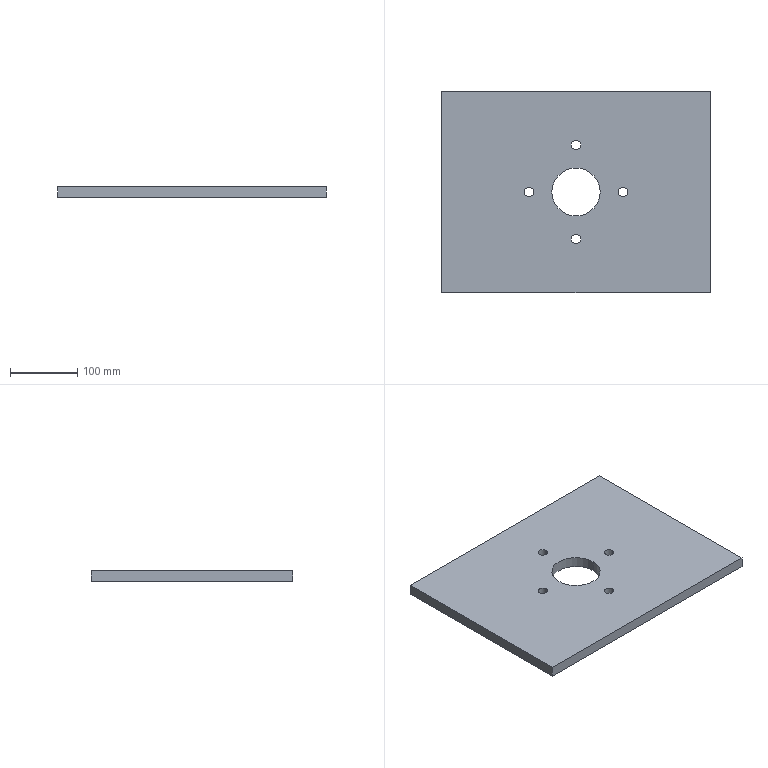Part | STEP file | 15-Steel plate | 1 solid | 16 faces | box 400 x 300 x 16 mm | volume 1845004 mm3 | cylinder 10 | plane 6 | commonest cylinder face diameters 14 x8 72 x2
STEP:
#1=CARTESIAN_POINT('',(0.,0.,0.));
#2=DIRECTION('',(0.,0.,1.));
#3=DIRECTION('',(1.,0.,0.));
#4=AXIS2_PLACEMENT_3D('',#1,#2,#3);
#5=CARTESIAN_POINT('',(207.,-80.,0.));
#6=VERTEX_POINT('',#5);
#7=CARTESIAN_POINT('',(207.,-80.,16.));
#8=VERTEX_POINT('',#7);
#9=CARTESIAN_POINT('',(207.,-80.,16.));
#10=DIRECTION('',(0.,0.,1.));
#11=VECTOR('',#10,1.);
#12=LINE('',#9,#11);
#13=CARTESIAN_POINT('',(200.,-80.,16.));
#14=DIRECTION('',(0.,0.,1.));
#15=DIRECTION('',(1.,0.,0.));
#16=AXIS2_PLACEMENT_3D('',#13,#14,#15);
#17=CYLINDRICAL_SURFACE('',#16,7.);
#18=CARTESIAN_POINT('',(6.283,0.));
#19=DIRECTION('',(0.,1.));
#20=VECTOR('',#19,1.);
#21=LINE('',#18,#20);
#22=(GEOMETRIC_REPRESENTATION_CONTEXT(2)PARAMETRIC_REPRESENTATION_CONTEXT()REPRESENTATION_CONTEXT('',''));
#23=DEFINITIONAL_REPRESENTATION('',(#21),#22);
#24=PCURVE('',#17,#23);
#25=CARTESIAN_POINT('',(200.,-80.,16.));
#26=DIRECTION('',(0.,0.,1.));
#27=DIRECTION('',(1.,0.,0.));
#28=AXIS2_PLACEMENT_3D('',#25,#26,#27);
#29=CYLINDRICAL_SURFACE('',#28,7.);
#30=CARTESIAN_POINT('',(0.,0.));
#31=DIRECTION('',(0.,1.));
#32=VECTOR('',#31,1.);
#33=LINE('',#30,#32);
#34=(GEOMETRIC_REPRESENTATION_CONTEXT(2)PARAMETRIC_REPRESENTATION_CONTEXT()REPRESENTATION_CONTEXT('',''));
#35=DEFINITIONAL_REPRESENTATION('',(#33),#34);
#36=PCURVE('',#29,#35);
#37=SURFACE_CURVE('',#12,(#24,#36),.PCURVE_S1.);
#38=EDGE_CURVE('',#6,#8,#37,.T.);
#39=ORIENTED_EDGE('',*,*,#38,.T.);
#40=CARTESIAN_POINT('',(193.,-80.,16.));
#41=VERTEX_POINT('',#40);
#42=CARTESIAN_POINT('',(200.,-80.,16.));
#43=DIRECTION('',(0.,0.,1.));
#44=DIRECTION('',(1.,0.,0.));
#45=AXIS2_PLACEMENT_3D('',#42,#43,#44);
#46=CIRCLE('',#45,7.);
#47=CARTESIAN_POINT('',(0.,0.));
#48=DIRECTION('',(1.,0.));
#49=VECTOR('',#48,1.);
#50=LINE('',#47,#49);
#51=(GEOMETRIC_REPRESENTATION_CONTEXT(2)PARAMETRIC_REPRESENTATION_CONTEXT()REPRESENTATION_CONTEXT('',''));
#52=DEFINITIONAL_REPRESENTATION('',(#50),#51);
#53=PCURVE('',#17,#52);
#54=CARTESIAN_POINT('',(0.,0.,16.));
#55=DIRECTION('',(0.,0.,1.));
#56=DIRECTION('',(1.,0.,0.));
#57=AXIS2_PLACEMENT_3D('',#54,#55,#56);
#58=PLANE('',#57);
#59=CARTESIAN_POINT('',(200.,-80.));
#60=DIRECTION('',(1.,0.));
#61=AXIS2_PLACEMENT_2D('',#59,#60);
#62=CIRCLE('',#61,7.);
#63=(GEOMETRIC_REPRESENTATION_CONTEXT(2)PARAMETRIC_REPRESENTATION_CONTEXT()REPRESENTATION_CONTEXT('',''));
#64=DEFINITIONAL_REPRESENTATION('',(#62),#63);
#65=PCURVE('',#58,#64);
#66=SURFACE_CURVE('',#46,(#53,#65),.PCURVE_S1.);
#67=EDGE_CURVE('',#41,#8,#66,.T.);
#68=ORIENTED_EDGE('',*,*,#67,.F.);
#69=CARTESIAN_POINT('',(193.,-80.,0.));
#70=VERTEX_POINT('',#69);
#71=CARTESIAN_POINT('',(193.,-80.,16.));
#72=DIRECTION('',(0.,0.,1.));
#73=VECTOR('',#72,1.);
#74=LINE('',#71,#73);
#75=CARTESIAN_POINT('',(3.142,0.));
#76=DIRECTION('',(0.,1.));
#77=VECTOR('',#76,1.);
#78=LINE('',#75,#77);
#79=(GEOMETRIC_REPRESENTATION_CONTEXT(2)PARAMETRIC_REPRESENTATION_CONTEXT()REPRESENTATION_CONTEXT('',''));
#80=DEFINITIONAL_REPRESENTATION('',(#78),#79);
#81=PCURVE('',#17,#80);
#82=CARTESIAN_POINT('',(3.142,0.));
#83=DIRECTION('',(0.,1.));
#84=VECTOR('',#83,1.);
#85=LINE('',#82,#84);
#86=(GEOMETRIC_REPRESENTATION_CONTEXT(2)PARAMETRIC_REPRESENTATION_CONTEXT()REPRESENTATION_CONTEXT('',''));
#87=DEFINITIONAL_REPRESENTATION('',(#85),#86);
#88=PCURVE('',#29,#87);
#89=SURFACE_CURVE('',#74,(#81,#88),.PCURVE_S1.);
#90=EDGE_CURVE('',#70,#41,#89,.T.);
#91=ORIENTED_EDGE('',*,*,#90,.F.);
#92=CARTESIAN_POINT('',(200.,-80.,0.));
#93=DIRECTION('',(0.,0.,1.));
#94=DIRECTION('',(1.,0.,0.));
#95=AXIS2_PLACEMENT_3D('',#92,#93,#94);
#96=CIRCLE('',#95,7.);
#97=CARTESIAN_POINT('',(0.,-16.));
#98=DIRECTION('',(1.,0.));
#99=VECTOR('',#98,1.);
#100=LINE('',#97,#99);
#101=(GEOMETRIC_REPRESENTATION_CONTEXT(2)PARAMETRIC_REPRESENTATION_CONTEXT()REPRESENTATION_CONTEXT('',''));
#102=DEFINITIONAL_REPRESENTATION('',(#100),#101);
#103=PCURVE('',#17,#102);
#104=CARTESIAN_POINT('',(0.,0.,0.));
#105=DIRECTION('',(0.,0.,1.));
#106=DIRECTION('',(1.,0.,0.));
#107=AXIS2_PLACEMENT_3D('',#104,#105,#106);
#108=PLANE('',#107);
#109=CARTESIAN_POINT('',(200.,-80.));
#110=DIRECTION('',(1.,0.));
#111=AXIS2_PLACEMENT_2D('',#109,#110);
#112=CIRCLE('',#111,7.);
#113=(GEOMETRIC_REPRESENTATION_CONTEXT(2)PARAMETRIC_REPRESENTATION_CONTEXT()REPRESENTATION_CONTEXT('',''));
#114=DEFINITIONAL_REPRESENTATION('',(#112),#113);
#115=PCURVE('',#108,#114);
#116=SURFACE_CURVE('',#96,(#103,#115),.PCURVE_S1.);
#117=EDGE_CURVE('',#70,#6,#116,.T.);
#118=ORIENTED_EDGE('',*,*,#117,.T.);
#119=EDGE_LOOP('',(#39,#68,#91,#118));
#120=FACE_BOUND('',#119,.F.);
#121=ADVANCED_FACE('',(#120),#17,.F.);
#122=CARTESIAN_POINT('',(207.,-220.,0.));
#123=VERTEX_POINT('',#122);
#124=CARTESIAN_POINT('',(207.,-220.,16.));
#125=VERTEX_POINT('',#124);
#126=CARTESIAN_POINT('',(207.,-220.,16.));
#127=DIRECTION('',(0.,0.,1.));
#128=VECTOR('',#127,1.);
#129=LINE('',#126,#128);
#130=CARTESIAN_POINT('',(200.,-220.,16.));
#131=DIRECTION('',(0.,0.,1.));
#132=DIRECTION('',(1.,0.,0.));
#133=AXIS2_PLACEMENT_3D('',#130,#131,#132);
#134=CYLINDRICAL_SURFACE('',#133,7.);
#135=CARTESIAN_POINT('',(6.283,0.));
#136=DIRECTION('',(0.,1.));
#137=VECTOR('',#136,1.);
#138=LINE('',#135,#137);
#139=(GEOMETRIC_REPRESENTATION_CONTEXT(2)PARAMETRIC_REPRESENTATION_CONTEXT()REPRESENTATION_CONTEXT('',''));
#140=DEFINITIONAL_REPRESENTATION('',(#138),#139);
#141=PCURVE('',#134,#140);
#142=CARTESIAN_POINT('',(200.,-220.,16.));
#143=DIRECTION('',(0.,0.,1.));
#144=DIRECTION('',(1.,0.,0.));
#145=AXIS2_PLACEMENT_3D('',#142,#143,#144);
#146=CYLINDRICAL_SURFACE('',#145,7.);
#147=CARTESIAN_POINT('',(0.,0.));
#148=DIRECTION('',(0.,1.));
#149=VECTOR('',#148,1.);
#150=LINE('',#147,#149);
#151=(GEOMETRIC_REPRESENTATION_CONTEXT(2)PARAMETRIC_REPRESENTATION_CONTEXT()REPRESENTATION_CONTEXT('',''));
#152=DEFINITIONAL_REPRESENTATION('',(#150),#151);
#153=PCURVE('',#146,#152);
#154=SURFACE_CURVE('',#129,(#141,#153),.PCURVE_S1.);
#155=EDGE_CURVE('',#123,#125,#154,.T.);
#156=ORIENTED_EDGE('',*,*,#155,.T.);
#157=CARTESIAN_POINT('',(193.,-220.,16.));
#158=VERTEX_POINT('',#157);
#159=CARTESIAN_POINT('',(200.,-220.,16.));
#160=DIRECTION('',(0.,0.,1.));
#161=DIRECTION('',(1.,0.,0.));
#162=AXIS2_PLACEMENT_3D('',#159,#160,#161);
#163=CIRCLE('',#162,7.);
#164=CARTESIAN_POINT('',(0.,0.));
#165=DIRECTION('',(1.,0.));
#166=VECTOR('',#165,1.);
#167=LINE('',#164,#166);
#168=(GEOMETRIC_REPRESENTATION_CONTEXT(2)PARAMETRIC_REPRESENTATION_CONTEXT()REPRESENTATION_CONTEXT('',''));
#169=DEFINITIONAL_REPRESENTATION('',(#167),#168);
#170=PCURVE('',#134,#169);
#171=CARTESIAN_POINT('',(200.,-220.));
#172=DIRECTION('',(1.,0.));
#173=AXIS2_PLACEMENT_2D('',#171,#172);
#174=CIRCLE('',#173,7.);
#175=(GEOMETRIC_REPRESENTATION_CONTEXT(2)PARAMETRIC_REPRESENTATION_CONTEXT()REPRESENTATION_CONTEXT('',''));
#176=DEFINITIONAL_REPRESENTATION('',(#174),#175);
#177=PCURVE('',#58,#176);
#178=SURFACE_CURVE('',#163,(#170,#177),.PCURVE_S1.);
#179=EDGE_CURVE('',#158,#125,#178,.T.);
#180=ORIENTED_EDGE('',*,*,#179,.F.);
#181=CARTESIAN_POINT('',(193.,-220.,0.));
#182=VERTEX_POINT('',#181);
#183=CARTESIAN_POINT('',(193.,-220.,16.));
#184=DIRECTION('',(0.,0.,1.));
#185=VECTOR('',#184,1.);
#186=LINE('',#183,#185);
#187=CARTESIAN_POINT('',(3.142,0.));
#188=DIRECTION('',(0.,1.));
#189=VECTOR('',#188,1.);
#190=LINE('',#187,#189);
#191=(GEOMETRIC_REPRESENTATION_CONTEXT(2)PARAMETRIC_REPRESENTATION_CONTEXT()REPRESENTATION_CONTEXT('',''));
#192=DEFINITIONAL_REPRESENTATION('',(#190),#191);
#193=PCURVE('',#134,#192);
#194=CARTESIAN_POINT('',(3.142,0.));
#195=DIRECTION('',(0.,1.));
#196=VECTOR('',#195,1.);
#197=LINE('',#194,#196);
#198=(GEOMETRIC_REPRESENTATION_CONTEXT(2)PARAMETRIC_REPRESENTATION_CONTEXT()REPRESENTATION_CONTEXT('',''));
#199=DEFINITIONAL_REPRESENTATION('',(#197),#198);
#200=PCURVE('',#146,#199);
#201=SURFACE_CURVE('',#186,(#193,#200),.PCURVE_S1.);
#202=EDGE_CURVE('',#182,#158,#201,.T.);
#203=ORIENTED_EDGE('',*,*,#202,.F.);
#204=CARTESIAN_POINT('',(200.,-220.,0.));
#205=DIRECTION('',(0.,0.,1.));
#206=DIRECTION('',(1.,0.,0.));
#207=AXIS2_PLACEMENT_3D('',#204,#205,#206);
#208=CIRCLE('',#207,7.);
#209=CARTESIAN_POINT('',(0.,-16.));
#210=DIRECTION('',(1.,0.));
#211=VECTOR('',#210,1.);
#212=LINE('',#209,#211);
#213=(GEOMETRIC_REPRESENTATION_CONTEXT(2)PARAMETRIC_REPRESENTATION_CONTEXT()REPRESENTATION_CONTEXT('',''));
#214=DEFINITIONAL_REPRESENTATION('',(#212),#213);
#215=PCURVE('',#134,#214);
#216=CARTESIAN_POINT('',(200.,-220.));
#217=DIRECTION('',(1.,0.));
#218=AXIS2_PLACEMENT_2D('',#216,#217);
#219=CIRCLE('',#218,7.);
#220=(GEOMETRIC_REPRESENTATION_CONTEXT(2)PARAMETRIC_REPRESENTATION_CONTEXT()REPRESENTATION_CONTEXT('',''));
#221=DEFINITIONAL_REPRESENTATION('',(#219),#220);
#222=PCURVE('',#108,#221);
#223=SURFACE_CURVE('',#208,(#215,#222),.PCURVE_S1.);
#224=EDGE_CURVE('',#182,#123,#223,.T.);
#225=ORIENTED_EDGE('',*,*,#224,.T.);
#226=EDGE_LOOP('',(#156,#180,#203,#225));
#227=FACE_BOUND('',#226,.F.);
#228=ADVANCED_FACE('',(#227),#134,.F.);
#229=CARTESIAN_POINT('',(277.,-150.,0.));
#230=VERTEX_POINT('',#229);
#231=CARTESIAN_POINT('',(277.,-150.,16.));
#232=VERTEX_POINT('',#231);
#233=CARTESIAN_POINT('',(277.,-150.,16.));
#234=DIRECTION('',(0.,0.,1.));
#235=VECTOR('',#234,1.);
#236=LINE('',#233,#235);
#237=CARTESIAN_POINT('',(270.,-150.,16.));
#238=DIRECTION('',(0.,0.,1.));
#239=DIRECTION('',(1.,0.,0.));
#240=AXIS2_PLACEMENT_3D('',#237,#238,#239);
#241=CYLINDRICAL_SURFACE('',#240,7.);
#242=CARTESIAN_POINT('',(6.283,0.));
#243=DIRECTION('',(0.,1.));
#244=VECTOR('',#243,1.);
#245=LINE('',#242,#244);
#246=(GEOMETRIC_REPRESENTATION_CONTEXT(2)PARAMETRIC_REPRESENTATION_CONTEXT()REPRESENTATION_CONTEXT('',''));
#247=DEFINITIONAL_REPRESENTATION('',(#245),#246);
#248=PCURVE('',#241,#247);
#249=CARTESIAN_POINT('',(270.,-150.,16.));
#250=DIRECTION('',(0.,0.,1.));
#251=DIRECTION('',(1.,0.,0.));
#252=AXIS2_PLACEMENT_3D('',#249,#250,#251);
#253=CYLINDRICAL_SURFACE('',#252,7.);
#254=CARTESIAN_POINT('',(0.,0.));
#255=DIRECTION('',(0.,1.));
#256=VECTOR('',#255,1.);
#257=LINE('',#254,#256);
#258=(GEOMETRIC_REPRESENTATION_CONTEXT(2)PARAMETRIC_REPRESENTATION_CONTEXT()REPRESENTATION_CONTEXT('',''));
#259=DEFINITIONAL_REPRESENTATION('',(#257),#258);
#260=PCURVE('',#253,#259);
#261=SURFACE_CURVE('',#236,(#248,#260),.PCURVE_S1.);
#262=EDGE_CURVE('',#230,#232,#261,.T.);
#263=ORIENTED_EDGE('',*,*,#262,.T.);
#264=CARTESIAN_POINT('',(263.,-150.,16.));
#265=VERTEX_POINT('',#264);
#266=CARTESIAN_POINT('',(270.,-150.,16.));
#267=DIRECTION('',(0.,0.,1.));
#268=DIRECTION('',(1.,0.,0.));
#269=AXIS2_PLACEMENT_3D('',#266,#267,#268);
#270=CIRCLE('',#269,7.);
#271=CARTESIAN_POINT('',(0.,0.));
#272=DIRECTION('',(1.,0.));
#273=VECTOR('',#272,1.);
#274=LINE('',#271,#273);
#275=(GEOMETRIC_REPRESENTATION_CONTEXT(2)PARAMETRIC_REPRESENTATION_CONTEXT()REPRESENTATION_CONTEXT('',''));
#276=DEFINITIONAL_REPRESENTATION('',(#274),#275);
#277=PCURVE('',#241,#276);
#278=CARTESIAN_POINT('',(270.,-150.));
#279=DIRECTION('',(1.,0.));
#280=AXIS2_PLACEMENT_2D('',#278,#279);
#281=CIRCLE('',#280,7.);
#282=(GEOMETRIC_REPRESENTATION_CONTEXT(2)PARAMETRIC_REPRESENTATION_CONTEXT()REPRESENTATION_CONTEXT('',''));
#283=DEFINITIONAL_REPRESENTATION('',(#281),#282);
#284=PCURVE('',#58,#283);
#285=SURFACE_CURVE('',#270,(#277,#284),.PCURVE_S1.);
#286=EDGE_CURVE('',#265,#232,#285,.T.);
#287=ORIENTED_EDGE('',*,*,#286,.F.);
#288=CARTESIAN_POINT('',(263.,-150.,0.));
#289=VERTEX_POINT('',#288);
#290=CARTESIAN_POINT('',(263.,-150.,16.));
#291=DIRECTION('',(0.,0.,1.));
#292=VECTOR('',#291,1.);
#293=LINE('',#290,#292);
#294=CARTESIAN_POINT('',(3.142,0.));
#295=DIRECTION('',(0.,1.));
#296=VECTOR('',#295,1.);
#297=LINE('',#294,#296);
#298=(GEOMETRIC_REPRESENTATION_CONTEXT(2)PARAMETRIC_REPRESENTATION_CONTEXT()REPRESENTATION_CONTEXT('',''));
#299=DEFINITIONAL_REPRESENTATION('',(#297),#298);
#300=PCURVE('',#241,#299);
#301=CARTESIAN_POINT('',(3.142,0.));
#302=DIRECTION('',(0.,1.));
#303=VECTOR('',#302,1.);
#304=LINE('',#301,#303);
#305=(GEOMETRIC_REPRESENTATION_CONTEXT(2)PARAMETRIC_REPRESENTATION_CONTEXT()REPRESENTATION_CONTEXT('',''));
#306=DEFINITIONAL_REPRESENTATION('',(#304),#305);
#307=PCURVE('',#253,#306);
#308=SURFACE_CURVE('',#293,(#300,#307),.PCURVE_S1.);
#309=EDGE_CURVE('',#289,#265,#308,.T.);
#310=ORIENTED_EDGE('',*,*,#309,.F.);
#311=CARTESIAN_POINT('',(270.,-150.,0.));
#312=DIRECTION('',(0.,0.,1.));
#313=DIRECTION('',(1.,0.,0.));
#314=AXIS2_PLACEMENT_3D('',#311,#312,#313);
#315=CIRCLE('',#314,7.);
#316=CARTESIAN_POINT('',(0.,-16.));
#317=DIRECTION('',(1.,0.));
#318=VECTOR('',#317,1.);
#319=LINE('',#316,#318);
#320=(GEOMETRIC_REPRESENTATION_CONTEXT(2)PARAMETRIC_REPRESENTATION_CONTEXT()REPRESENTATION_CONTEXT('',''));
#321=DEFINITIONAL_REPRESENTATION('',(#319),#320);
#322=PCURVE('',#241,#321);
#323=CARTESIAN_POINT('',(270.,-150.));
#324=DIRECTION('',(1.,0.));
#325=AXIS2_PLACEMENT_2D('',#323,#324);
#326=CIRCLE('',#325,7.);
#327=(GEOMETRIC_REPRESENTATION_CONTEXT(2)PARAMETRIC_REPRESENTATION_CONTEXT()REPRESENTATION_CONTEXT('',''));
#328=DEFINITIONAL_REPRESENTATION('',(#326),#327);
#329=PCURVE('',#108,#328);
#330=SURFACE_CURVE('',#315,(#322,#329),.PCURVE_S1.);
#331=EDGE_CURVE('',#289,#230,#330,.T.);
#332=ORIENTED_EDGE('',*,*,#331,.T.);
#333=EDGE_LOOP('',(#263,#287,#310,#332));
#334=FACE_BOUND('',#333,.F.);
#335=ADVANCED_FACE('',(#334),#241,.F.);
#336=CARTESIAN_POINT('',(137.,-150.,0.));
#337=VERTEX_POINT('',#336);
#338=CARTESIAN_POINT('',(137.,-150.,16.));
#339=VERTEX_POINT('',#338);
#340=CARTESIAN_POINT('',(137.,-150.,16.));
#341=DIRECTION('',(0.,0.,1.));
#342=VECTOR('',#341,1.);
#343=LINE('',#340,#342);
#344=CARTESIAN_POINT('',(130.,-150.,16.));
#345=DIRECTION('',(0.,0.,1.));
#346=DIRECTION('',(1.,0.,0.));
#347=AXIS2_PLACEMENT_3D('',#344,#345,#346);
#348=CYLINDRICAL_SURFACE('',#347,7.);
#349=CARTESIAN_POINT('',(6.283,0.));
#350=DIRECTION('',(0.,1.));
#351=VECTOR('',#350,1.);
#352=LINE('',#349,#351);
#353=(GEOMETRIC_REPRESENTATION_CONTEXT(2)PARAMETRIC_REPRESENTATION_CONTEXT()REPRESENTATION_CONTEXT('',''));
#354=DEFINITIONAL_REPRESENTATION('',(#352),#353);
#355=PCURVE('',#348,#354);
#356=CARTESIAN_POINT('',(130.,-150.,16.));
#357=DIRECTION('',(0.,0.,1.));
#358=DIRECTION('',(1.,0.,0.));
#359=AXIS2_PLACEMENT_3D('',#356,#357,#358);
#360=CYLINDRICAL_SURFACE('',#359,7.);
#361=CARTESIAN_POINT('',(0.,0.));
#362=DIRECTION('',(0.,1.));
#363=VECTOR('',#362,1.);
#364=LINE('',#361,#363);
#365=(GEOMETRIC_REPRESENTATION_CONTEXT(2)PARAMETRIC_REPRESENTATION_CONTEXT()REPRESENTATION_CONTEXT('',''));
#366=DEFINITIONAL_REPRESENTATION('',(#364),#365);
#367=PCURVE('',#360,#366);
#368=SURFACE_CURVE('',#343,(#355,#367),.PCURVE_S1.);
#369=EDGE_CURVE('',#337,#339,#368,.T.);
#370=ORIENTED_EDGE('',*,*,#369,.T.);
#371=CARTESIAN_POINT('',(123.,-150.,16.));
#372=VERTEX_POINT('',#371);
#373=CARTESIAN_POINT('',(130.,-150.,16.));
#374=DIRECTION('',(0.,0.,1.));
#375=DIRECTION('',(1.,0.,0.));
#376=AXIS2_PLACEMENT_3D('',#373,#374,#375);
#377=CIRCLE('',#376,7.);
#378=CARTESIAN_POINT('',(0.,0.));
#379=DIRECTION('',(1.,0.));
#380=VECTOR('',#379,1.);
#381=LINE('',#378,#380);
#382=(GEOMETRIC_REPRESENTATION_CONTEXT(2)PARAMETRIC_REPRESENTATION_CONTEXT()REPRESENTATION_CONTEXT('',''));
#383=DEFINITIONAL_REPRESENTATION('',(#381),#382);
#384=PCURVE('',#348,#383);
#385=CARTESIAN_POINT('',(130.,-150.));
#386=DIRECTION('',(1.,0.));
#387=AXIS2_PLACEMENT_2D('',#385,#386);
#388=CIRCLE('',#387,7.);
#389=(GEOMETRIC_REPRESENTATION_CONTEXT(2)PARAMETRIC_REPRESENTATION_CONTEXT()REPRESENTATION_CONTEXT('',''));
#390=DEFINITIONAL_REPRESENTATION('',(#388),#389);
#391=PCURVE('',#58,#390);
#392=SURFACE_CURVE('',#377,(#384,#391),.PCURVE_S1.);
#393=EDGE_CURVE('',#372,#339,#392,.T.);
#394=ORIENTED_EDGE('',*,*,#393,.F.);
#395=CARTESIAN_POINT('',(123.,-150.,0.));
#396=VERTEX_POINT('',#395);
#397=CARTESIAN_POINT('',(123.,-150.,16.));
#398=DIRECTION('',(0.,0.,1.));
#399=VECTOR('',#398,1.);
#400=LINE('',#397,#399);
#401=CARTESIAN_POINT('',(3.142,0.));
#402=DIRECTION('',(0.,1.));
#403=VECTOR('',#402,1.);
#404=LINE('',#401,#403);
#405=(GEOMETRIC_REPRESENTATION_CONTEXT(2)PARAMETRIC_REPRESENTATION_CONTEXT()REPRESENTATION_CONTEXT('',''));
#406=DEFINITIONAL_REPRESENTATION('',(#404),#405);
#407=PCURVE('',#348,#406);
#408=CARTESIAN_POINT('',(3.142,0.));
#409=DIRECTION('',(0.,1.));
#410=VECTOR('',#409,1.);
#411=LINE('',#408,#410);
#412=(GEOMETRIC_REPRESENTATION_CONTEXT(2)PARAMETRIC_REPRESENTATION_CONTEXT()REPRESENTATION_CONTEXT('',''));
#413=DEFINITIONAL_REPRESENTATION('',(#411),#412);
#414=PCURVE('',#360,#413);
#415=SURFACE_CURVE('',#400,(#407,#414),.PCURVE_S1.);
#416=EDGE_CURVE('',#396,#372,#415,.T.);
#417=ORIENTED_EDGE('',*,*,#416,.F.);
#418=CARTESIAN_POINT('',(130.,-150.,0.));
#419=DIRECTION('',(0.,0.,1.));
#420=DIRECTION('',(1.,0.,0.));
#421=AXIS2_PLACEMENT_3D('',#418,#419,#420);
#422=CIRCLE('',#421,7.);
#423=CARTESIAN_POINT('',(0.,-16.));
#424=DIRECTION('',(1.,0.));
#425=VECTOR('',#424,1.);
#426=LINE('',#423,#425);
#427=(GEOMETRIC_REPRESENTATION_CONTEXT(2)PARAMETRIC_REPRESENTATION_CONTEXT()REPRESENTATION_CONTEXT('',''));
#428=DEFINITIONAL_REPRESENTATION('',(#426),#427);
#429=PCURVE('',#348,#428);
#430=CARTESIAN_POINT('',(130.,-150.));
#431=DIRECTION('',(1.,0.));
#432=AXIS2_PLACEMENT_2D('',#430,#431);
#433=CIRCLE('',#432,7.);
#434=(GEOMETRIC_REPRESENTATION_CONTEXT(2)PARAMETRIC_REPRESENTATION_CONTEXT()REPRESENTATION_CONTEXT('',''));
#435=DEFINITIONAL_REPRESENTATION('',(#433),#434);
#436=PCURVE('',#108,#435);
#437=SURFACE_CURVE('',#422,(#429,#436),.PCURVE_S1.);
#438=EDGE_CURVE('',#396,#337,#437,.T.);
#439=ORIENTED_EDGE('',*,*,#438,.T.);
#440=EDGE_LOOP('',(#370,#394,#417,#439));
#441=FACE_BOUND('',#440,.F.);
#442=ADVANCED_FACE('',(#441),#348,.F.);
#443=CARTESIAN_POINT('',(164.,-150.,16.));
#444=VERTEX_POINT('',#443);
#445=CARTESIAN_POINT('',(164.,-150.,0.));
#446=VERTEX_POINT('',#445);
#447=CARTESIAN_POINT('',(164.,-150.,16.));
#448=DIRECTION('',(0.,0.,-1.));
#449=VECTOR('',#448,1.);
#450=LINE('',#447,#449);
#451=CARTESIAN_POINT('',(200.,-150.,16.));
#452=DIRECTION('',(0.,0.,-1.));
#453=DIRECTION('',(-1.,0.,0.));
#454=AXIS2_PLACEMENT_3D('',#451,#452,#453);
#455=CYLINDRICAL_SURFACE('',#454,36.);
#456=CARTESIAN_POINT('',(6.283,0.));
#457=DIRECTION('',(0.,1.));
#458=VECTOR('',#457,1.);
#459=LINE('',#456,#458);
#460=(GEOMETRIC_REPRESENTATION_CONTEXT(2)PARAMETRIC_REPRESENTATION_CONTEXT()REPRESENTATION_CONTEXT('',''));
#461=DEFINITIONAL_REPRESENTATION('',(#459),#460);
#462=PCURVE('',#455,#461);
#463=CARTESIAN_POINT('',(200.,-150.,16.));
#464=DIRECTION('',(0.,0.,-1.));
#465=DIRECTION('',(-1.,0.,0.));
#466=AXIS2_PLACEMENT_3D('',#463,#464,#465);
#467=CYLINDRICAL_SURFACE('',#466,36.);
#468=CARTESIAN_POINT('',(0.,0.));
#469=DIRECTION('',(0.,1.));
#470=VECTOR('',#469,1.);
#471=LINE('',#468,#470);
#472=(GEOMETRIC_REPRESENTATION_CONTEXT(2)PARAMETRIC_REPRESENTATION_CONTEXT()REPRESENTATION_CONTEXT('',''));
#473=DEFINITIONAL_REPRESENTATION('',(#471),#472);
#474=PCURVE('',#467,#473);
#475=SURFACE_CURVE('',#450,(#462,#474),.PCURVE_S1.);
#476=EDGE_CURVE('',#444,#446,#475,.T.);
#477=ORIENTED_EDGE('',*,*,#476,.T.);
#478=CARTESIAN_POINT('',(236.,-150.,0.));
#479=VERTEX_POINT('',#478);
#480=CARTESIAN_POINT('',(200.,-150.,0.));
#481=DIRECTION('',(0.,0.,1.));
#482=DIRECTION('',(1.,0.,0.));
#483=AXIS2_PLACEMENT_3D('',#480,#481,#482);
#484=CIRCLE('',#483,36.);
#485=CARTESIAN_POINT('',(9.425,16.));
#486=DIRECTION('',(-1.,0.));
#487=VECTOR('',#486,1.);
#488=LINE('',#485,#487);
#489=(GEOMETRIC_REPRESENTATION_CONTEXT(2)PARAMETRIC_REPRESENTATION_CONTEXT()REPRESENTATION_CONTEXT('',''));
#490=DEFINITIONAL_REPRESENTATION('',(#488),#489);
#491=PCURVE('',#455,#490);
#492=CARTESIAN_POINT('',(200.,-150.));
#493=DIRECTION('',(1.,0.));
#494=AXIS2_PLACEMENT_2D('',#492,#493);
#495=CIRCLE('',#494,36.);
#496=(GEOMETRIC_REPRESENTATION_CONTEXT(2)PARAMETRIC_REPRESENTATION_CONTEXT()REPRESENTATION_CONTEXT('',''));
#497=DEFINITIONAL_REPRESENTATION('',(#495),#496);
#498=PCURVE('',#108,#497);
#499=SURFACE_CURVE('',#484,(#491,#498),.PCURVE_S1.);
#500=EDGE_CURVE('',#446,#479,#499,.T.);
#501=ORIENTED_EDGE('',*,*,#500,.T.);
#502=CARTESIAN_POINT('',(236.,-150.,16.));
#503=VERTEX_POINT('',#502);
#504=CARTESIAN_POINT('',(236.,-150.,16.));
#505=DIRECTION('',(0.,0.,-1.));
#506=VECTOR('',#505,1.);
#507=LINE('',#504,#506);
#508=CARTESIAN_POINT('',(3.142,0.));
#509=DIRECTION('',(0.,1.));
#510=VECTOR('',#509,1.);
#511=LINE('',#508,#510);
#512=(GEOMETRIC_REPRESENTATION_CONTEXT(2)PARAMETRIC_REPRESENTATION_CONTEXT()REPRESENTATION_CONTEXT('',''));
#513=DEFINITIONAL_REPRESENTATION('',(#511),#512);
#514=PCURVE('',#455,#513);
#515=CARTESIAN_POINT('',(3.142,0.));
#516=DIRECTION('',(0.,1.));
#517=VECTOR('',#516,1.);
#518=LINE('',#515,#517);
#519=(GEOMETRIC_REPRESENTATION_CONTEXT(2)PARAMETRIC_REPRESENTATION_CONTEXT()REPRESENTATION_CONTEXT('',''));
#520=DEFINITIONAL_REPRESENTATION('',(#518),#519);
#521=PCURVE('',#467,#520);
#522=SURFACE_CURVE('',#507,(#514,#521),.PCURVE_S1.);
#523=EDGE_CURVE('',#503,#479,#522,.T.);
#524=ORIENTED_EDGE('',*,*,#523,.F.);
#525=CARTESIAN_POINT('',(200.,-150.,16.));
#526=DIRECTION('',(0.,0.,1.));
#527=DIRECTION('',(1.,0.,0.));
#528=AXIS2_PLACEMENT_3D('',#525,#526,#527);
#529=CIRCLE('',#528,36.);
#530=CARTESIAN_POINT('',(9.425,0.));
#531=DIRECTION('',(-1.,0.));
#532=VECTOR('',#531,1.);
#533=LINE('',#530,#532);
#534=(GEOMETRIC_REPRESENTATION_CONTEXT(2)PARAMETRIC_REPRESENTATION_CONTEXT()REPRESENTATION_CONTEXT('',''));
#535=DEFINITIONAL_REPRESENTATION('',(#533),#534);
#536=PCURVE('',#455,#535);
#537=CARTESIAN_POINT('',(200.,-150.));
#538=DIRECTION('',(1.,0.));
#539=AXIS2_PLACEMENT_2D('',#537,#538);
#540=CIRCLE('',#539,36.);
#541=(GEOMETRIC_REPRESENTATION_CONTEXT(2)PARAMETRIC_REPRESENTATION_CONTEXT()REPRESENTATION_CONTEXT('',''));
#542=DEFINITIONAL_REPRESENTATION('',(#540),#541);
#543=PCURVE('',#58,#542);
#544=SURFACE_CURVE('',#529,(#536,#543),.PCURVE_S1.);
#545=EDGE_CURVE('',#444,#503,#544,.T.);
#546=ORIENTED_EDGE('',*,*,#545,.F.);
#547=EDGE_LOOP('',(#477,#501,#524,#546));
#548=FACE_BOUND('',#547,.F.);
#549=ADVANCED_FACE('',(#548),#455,.F.);
#550=CARTESIAN_POINT('',(200.,-80.,16.));
#551=DIRECTION('',(0.,0.,1.));
#552=DIRECTION('',(1.,0.,0.));
#553=AXIS2_PLACEMENT_3D('',#550,#551,#552);
#554=CIRCLE('',#553,7.);
#555=CARTESIAN_POINT('',(200.,-80.));
#556=DIRECTION('',(1.,0.));
#557=AXIS2_PLACEMENT_2D('',#555,#556);
#558=CIRCLE('',#557,7.);
#559=(GEOMETRIC_REPRESENTATION_CONTEXT(2)PARAMETRIC_REPRESENTATION_CONTEXT()REPRESENTATION_CONTEXT('',''));
#560=DEFINITIONAL_REPRESENTATION('',(#558),#559);
#561=PCURVE('',#58,#560);
#562=CARTESIAN_POINT('',(0.,0.));
#563=DIRECTION('',(1.,0.));
#564=VECTOR('',#563,1.);
#565=LINE('',#562,#564);
#566=(GEOMETRIC_REPRESENTATION_CONTEXT(2)PARAMETRIC_REPRESENTATION_CONTEXT()REPRESENTATION_CONTEXT('',''));
#567=DEFINITIONAL_REPRESENTATION('',(#565),#566);
#568=PCURVE('',#29,#567);
#569=SURFACE_CURVE('',#554,(#561,#568),.PCURVE_S1.);
#570=EDGE_CURVE('',#8,#41,#569,.T.);
#571=ORIENTED_EDGE('',*,*,#570,.F.);
#572=ORIENTED_EDGE('',*,*,#67,.F.);
#573=EDGE_LOOP('',(#571,#572));
#574=FACE_BOUND('',#573,.T.);
#575=CARTESIAN_POINT('',(200.,-220.,16.));
#576=DIRECTION('',(0.,0.,1.));
#577=DIRECTION('',(1.,0.,0.));
#578=AXIS2_PLACEMENT_3D('',#575,#576,#577);
#579=CIRCLE('',#578,7.);
#580=CARTESIAN_POINT('',(200.,-220.));
#581=DIRECTION('',(1.,0.));
#582=AXIS2_PLACEMENT_2D('',#580,#581);
#583=CIRCLE('',#582,7.);
#584=(GEOMETRIC_REPRESENTATION_CONTEXT(2)PARAMETRIC_REPRESENTATION_CONTEXT()REPRESENTATION_CONTEXT('',''));
#585=DEFINITIONAL_REPRESENTATION('',(#583),#584);
#586=PCURVE('',#58,#585);
#587=CARTESIAN_POINT('',(0.,0.));
#588=DIRECTION('',(1.,0.));
#589=VECTOR('',#588,1.);
#590=LINE('',#587,#589);
#591=(GEOMETRIC_REPRESENTATION_CONTEXT(2)PARAMETRIC_REPRESENTATION_CONTEXT()REPRESENTATION_CONTEXT('',''));
#592=DEFINITIONAL_REPRESENTATION('',(#590),#591);
#593=PCURVE('',#146,#592);
#594=SURFACE_CURVE('',#579,(#586,#593),.PCURVE_S1.);
#595=EDGE_CURVE('',#125,#158,#594,.T.);
#596=ORIENTED_EDGE('',*,*,#595,.F.);
#597=ORIENTED_EDGE('',*,*,#179,.F.);
#598=EDGE_LOOP('',(#596,#597));
#599=FACE_BOUND('',#598,.T.);
#600=CARTESIAN_POINT('',(270.,-150.,16.));
#601=DIRECTION('',(0.,0.,1.));
#602=DIRECTION('',(1.,0.,0.));
#603=AXIS2_PLACEMENT_3D('',#600,#601,#602);
#604=CIRCLE('',#603,7.);
#605=CARTESIAN_POINT('',(270.,-150.));
#606=DIRECTION('',(1.,0.));
#607=AXIS2_PLACEMENT_2D('',#605,#606);
#608=CIRCLE('',#607,7.);
#609=(GEOMETRIC_REPRESENTATION_CONTEXT(2)PARAMETRIC_REPRESENTATION_CONTEXT()REPRESENTATION_CONTEXT('',''));
#610=DEFINITIONAL_REPRESENTATION('',(#608),#609);
#611=PCURVE('',#58,#610);
#612=CARTESIAN_POINT('',(0.,0.));
#613=DIRECTION('',(1.,0.));
#614=VECTOR('',#613,1.);
#615=LINE('',#612,#614);
#616=(GEOMETRIC_REPRESENTATION_CONTEXT(2)PARAMETRIC_REPRESENTATION_CONTEXT()REPRESENTATION_CONTEXT('',''));
#617=DEFINITIONAL_REPRESENTATION('',(#615),#616);
#618=PCURVE('',#253,#617);
#619=SURFACE_CURVE('',#604,(#611,#618),.PCURVE_S1.);
#620=EDGE_CURVE('',#232,#265,#619,.T.);
#621=ORIENTED_EDGE('',*,*,#620,.F.);
#622=ORIENTED_EDGE('',*,*,#286,.F.);
#623=EDGE_LOOP('',(#621,#622));
#624=FACE_BOUND('',#623,.T.);
#625=CARTESIAN_POINT('',(130.,-150.,16.));
#626=DIRECTION('',(0.,0.,1.));
#627=DIRECTION('',(1.,0.,0.));
#628=AXIS2_PLACEMENT_3D('',#625,#626,#627);
#629=CIRCLE('',#628,7.);
#630=CARTESIAN_POINT('',(130.,-150.));
#631=DIRECTION('',(1.,0.));
#632=AXIS2_PLACEMENT_2D('',#630,#631);
#633=CIRCLE('',#632,7.);
#634=(GEOMETRIC_REPRESENTATION_CONTEXT(2)PARAMETRIC_REPRESENTATION_CONTEXT()REPRESENTATION_CONTEXT('',''));
#635=DEFINITIONAL_REPRESENTATION('',(#633),#634);
#636=PCURVE('',#58,#635);
#637=CARTESIAN_POINT('',(0.,0.));
#638=DIRECTION('',(1.,0.));
#639=VECTOR('',#638,1.);
#640=LINE('',#637,#639);
#641=(GEOMETRIC_REPRESENTATION_CONTEXT(2)PARAMETRIC_REPRESENTATION_CONTEXT()REPRESENTATION_CONTEXT('',''));
#642=DEFINITIONAL_REPRESENTATION('',(#640),#641);
#643=PCURVE('',#360,#642);
#644=SURFACE_CURVE('',#629,(#636,#643),.PCURVE_S1.);
#645=EDGE_CURVE('',#339,#372,#644,.T.);
#646=ORIENTED_EDGE('',*,*,#645,.F.);
#647=ORIENTED_EDGE('',*,*,#393,.F.);
#648=EDGE_LOOP('',(#646,#647));
#649=FACE_BOUND('',#648,.T.);
#650=CARTESIAN_POINT('',(0.,0.,16.));
#651=VERTEX_POINT('',#650);
#652=CARTESIAN_POINT('',(0.,-300.,16.));
#653=VERTEX_POINT('',#652);
#654=CARTESIAN_POINT('',(0.,0.,16.));
#655=DIRECTION('',(0.,-1.,0.));
#656=VECTOR('',#655,1.);
#657=LINE('',#654,#656);
#658=CARTESIAN_POINT('',(0.,0.));
#659=DIRECTION('',(0.,-1.));
#660=VECTOR('',#659,1.);
#661=LINE('',#658,#660);
#662=(GEOMETRIC_REPRESENTATION_CONTEXT(2)PARAMETRIC_REPRESENTATION_CONTEXT()REPRESENTATION_CONTEXT('',''));
#663=DEFINITIONAL_REPRESENTATION('',(#661),#662);
#664=PCURVE('',#58,#663);
#665=CARTESIAN_POINT('',(0.,0.,16.));
#666=DIRECTION('',(1.,0.,0.));
#667=DIRECTION('',(0.,1.,0.));
#668=AXIS2_PLACEMENT_3D('',#665,#666,#667);
#669=PLANE('',#668);
#670=CARTESIAN_POINT('',(0.,0.));
#671=DIRECTION('',(-1.,0.));
#672=VECTOR('',#671,1.);
#673=LINE('',#670,#672);
#674=(GEOMETRIC_REPRESENTATION_CONTEXT(2)PARAMETRIC_REPRESENTATION_CONTEXT()REPRESENTATION_CONTEXT('',''));
#675=DEFINITIONAL_REPRESENTATION('',(#673),#674);
#676=PCURVE('',#669,#675);
#677=SURFACE_CURVE('',#657,(#664,#676),.PCURVE_S1.);
#678=EDGE_CURVE('',#651,#653,#677,.T.);
#679=ORIENTED_EDGE('',*,*,#678,.T.);
#680=CARTESIAN_POINT('',(400.,-300.,16.));
#681=VERTEX_POINT('',#680);
#682=CARTESIAN_POINT('',(0.,-300.,16.));
#683=DIRECTION('',(1.,0.,0.));
#684=VECTOR('',#683,1.);
#685=LINE('',#682,#684);
#686=CARTESIAN_POINT('',(0.,-300.));
#687=DIRECTION('',(1.,0.));
#688=VECTOR('',#687,1.);
#689=LINE('',#686,#688);
#690=(GEOMETRIC_REPRESENTATION_CONTEXT(2)PARAMETRIC_REPRESENTATION_CONTEXT()REPRESENTATION_CONTEXT('',''));
#691=DEFINITIONAL_REPRESENTATION('',(#689),#690);
#692=PCURVE('',#58,#691);
#693=CARTESIAN_POINT('',(0.,-300.,16.));
#694=DIRECTION('',(0.,1.,0.));
#695=DIRECTION('',(0.,0.,1.));
#696=AXIS2_PLACEMENT_3D('',#693,#694,#695);
#697=PLANE('',#696);
#698=CARTESIAN_POINT('',(0.,0.));
#699=DIRECTION('',(0.,1.));
#700=VECTOR('',#699,1.);
#701=LINE('',#698,#700);
#702=(GEOMETRIC_REPRESENTATION_CONTEXT(2)PARAMETRIC_REPRESENTATION_CONTEXT()REPRESENTATION_CONTEXT('',''));
#703=DEFINITIONAL_REPRESENTATION('',(#701),#702);
#704=PCURVE('',#697,#703);
#705=SURFACE_CURVE('',#685,(#692,#704),.PCURVE_S1.);
#706=EDGE_CURVE('',#653,#681,#705,.T.);
#707=ORIENTED_EDGE('',*,*,#706,.T.);
#708=CARTESIAN_POINT('',(400.,0.,16.));
#709=VERTEX_POINT('',#708);
#710=CARTESIAN_POINT('',(400.,0.,16.));
#711=DIRECTION('',(0.,1.,0.));
#712=VECTOR('',#711,1.);
#713=LINE('',#710,#712);
#714=CARTESIAN_POINT('',(400.,0.));
#715=DIRECTION('',(0.,1.));
#716=VECTOR('',#715,1.);
#717=LINE('',#714,#716);
#718=(GEOMETRIC_REPRESENTATION_CONTEXT(2)PARAMETRIC_REPRESENTATION_CONTEXT()REPRESENTATION_CONTEXT('',''));
#719=DEFINITIONAL_REPRESENTATION('',(#717),#718);
#720=PCURVE('',#58,#719);
#721=CARTESIAN_POINT('',(400.,0.,16.));
#722=DIRECTION('',(-1.,0.,0.));
#723=DIRECTION('',(0.,-1.,0.));
#724=AXIS2_PLACEMENT_3D('',#721,#722,#723);
#725=PLANE('',#724);
#726=CARTESIAN_POINT('',(0.,0.));
#727=DIRECTION('',(-1.,0.));
#728=VECTOR('',#727,1.);
#729=LINE('',#726,#728);
#730=(GEOMETRIC_REPRESENTATION_CONTEXT(2)PARAMETRIC_REPRESENTATION_CONTEXT()REPRESENTATION_CONTEXT('',''));
#731=DEFINITIONAL_REPRESENTATION('',(#729),#730);
#732=PCURVE('',#725,#731);
#733=SURFACE_CURVE('',#713,(#720,#732),.PCURVE_S1.);
#734=EDGE_CURVE('',#681,#709,#733,.T.);
#735=ORIENTED_EDGE('',*,*,#734,.T.);
#736=CARTESIAN_POINT('',(0.,0.,16.));
#737=DIRECTION('',(-1.,0.,0.));
#738=VECTOR('',#737,1.);
#739=LINE('',#736,#738);
#740=CARTESIAN_POINT('',(0.,0.));
#741=DIRECTION('',(-1.,0.));
#742=VECTOR('',#741,1.);
#743=LINE('',#740,#742);
#744=(GEOMETRIC_REPRESENTATION_CONTEXT(2)PARAMETRIC_REPRESENTATION_CONTEXT()REPRESENTATION_CONTEXT('',''));
#745=DEFINITIONAL_REPRESENTATION('',(#743),#744);
#746=PCURVE('',#58,#745);
#747=CARTESIAN_POINT('',(0.,0.,16.));
#748=DIRECTION('',(0.,-1.,0.));
#749=DIRECTION('',(0.,0.,-1.));
#750=AXIS2_PLACEMENT_3D('',#747,#748,#749);
#751=PLANE('',#750);
#752=CARTESIAN_POINT('',(0.,0.));
#753=DIRECTION('',(0.,-1.));
#754=VECTOR('',#753,1.);
#755=LINE('',#752,#754);
#756=(GEOMETRIC_REPRESENTATION_CONTEXT(2)PARAMETRIC_REPRESENTATION_CONTEXT()REPRESENTATION_CONTEXT('',''));
#757=DEFINITIONAL_REPRESENTATION('',(#755),#756);
#758=PCURVE('',#751,#757);
#759=SURFACE_CURVE('',#739,(#746,#758),.PCURVE_S1.);
#760=EDGE_CURVE('',#709,#651,#759,.T.);
#761=ORIENTED_EDGE('',*,*,#760,.T.);
#762=EDGE_LOOP('',(#679,#707,#735,#761));
#763=FACE_BOUND('',#762,.T.);
#764=ORIENTED_EDGE('',*,*,#545,.F.);
#765=CARTESIAN_POINT('',(200.,-150.,16.));
#766=DIRECTION('',(0.,0.,1.));
#767=DIRECTION('',(1.,0.,0.));
#768=AXIS2_PLACEMENT_3D('',#765,#766,#767);
#769=CIRCLE('',#768,36.);
#770=CARTESIAN_POINT('',(200.,-150.));
#771=DIRECTION('',(1.,0.));
#772=AXIS2_PLACEMENT_2D('',#770,#771);
#773=CIRCLE('',#772,36.);
#774=(GEOMETRIC_REPRESENTATION_CONTEXT(2)PARAMETRIC_REPRESENTATION_CONTEXT()REPRESENTATION_CONTEXT('',''));
#775=DEFINITIONAL_REPRESENTATION('',(#773),#774);
#776=PCURVE('',#58,#775);
#777=CARTESIAN_POINT('',(3.142,0.));
#778=DIRECTION('',(-1.,0.));
#779=VECTOR('',#778,1.);
#780=LINE('',#777,#779);
#781=(GEOMETRIC_REPRESENTATION_CONTEXT(2)PARAMETRIC_REPRESENTATION_CONTEXT()REPRESENTATION_CONTEXT('',''));
#782=DEFINITIONAL_REPRESENTATION('',(#780),#781);
#783=PCURVE('',#467,#782);
#784=SURFACE_CURVE('',#769,(#776,#783),.PCURVE_S1.);
#785=EDGE_CURVE('',#503,#444,#784,.T.);
#786=ORIENTED_EDGE('',*,*,#785,.F.);
#787=EDGE_LOOP('',(#764,#786));
#788=FACE_BOUND('',#787,.T.);
#789=ADVANCED_FACE('',(#574,#599,#624,#649,#763,#788),#58,.T.);
#790=CARTESIAN_POINT('',(200.,-80.,0.));
#791=DIRECTION('',(0.,0.,1.));
#792=DIRECTION('',(1.,0.,0.));
#793=AXIS2_PLACEMENT_3D('',#790,#791,#792);
#794=CIRCLE('',#793,7.);
#795=CARTESIAN_POINT('',(200.,-80.));
#796=DIRECTION('',(1.,0.));
#797=AXIS2_PLACEMENT_2D('',#795,#796);
#798=CIRCLE('',#797,7.);
#799=(GEOMETRIC_REPRESENTATION_CONTEXT(2)PARAMETRIC_REPRESENTATION_CONTEXT()REPRESENTATION_CONTEXT('',''));
#800=DEFINITIONAL_REPRESENTATION('',(#798),#799);
#801=PCURVE('',#108,#800);
#802=CARTESIAN_POINT('',(0.,-16.));
#803=DIRECTION('',(1.,0.));
#804=VECTOR('',#803,1.);
#805=LINE('',#802,#804);
#806=(GEOMETRIC_REPRESENTATION_CONTEXT(2)PARAMETRIC_REPRESENTATION_CONTEXT()REPRESENTATION_CONTEXT('',''));
#807=DEFINITIONAL_REPRESENTATION('',(#805),#806);
#808=PCURVE('',#29,#807);
#809=SURFACE_CURVE('',#794,(#801,#808),.PCURVE_S1.);
#810=EDGE_CURVE('',#6,#70,#809,.T.);
#811=ORIENTED_EDGE('',*,*,#810,.T.);
#812=ORIENTED_EDGE('',*,*,#117,.T.);
#813=EDGE_LOOP('',(#811,#812));
#814=FACE_BOUND('',#813,.T.);
#815=CARTESIAN_POINT('',(200.,-220.,0.));
#816=DIRECTION('',(0.,0.,1.));
#817=DIRECTION('',(1.,0.,0.));
#818=AXIS2_PLACEMENT_3D('',#815,#816,#817);
#819=CIRCLE('',#818,7.);
#820=CARTESIAN_POINT('',(200.,-220.));
#821=DIRECTION('',(1.,0.));
#822=AXIS2_PLACEMENT_2D('',#820,#821);
#823=CIRCLE('',#822,7.);
#824=(GEOMETRIC_REPRESENTATION_CONTEXT(2)PARAMETRIC_REPRESENTATION_CONTEXT()REPRESENTATION_CONTEXT('',''));
#825=DEFINITIONAL_REPRESENTATION('',(#823),#824);
#826=PCURVE('',#108,#825);
#827=CARTESIAN_POINT('',(0.,-16.));
#828=DIRECTION('',(1.,0.));
#829=VECTOR('',#828,1.);
#830=LINE('',#827,#829);
#831=(GEOMETRIC_REPRESENTATION_CONTEXT(2)PARAMETRIC_REPRESENTATION_CONTEXT()REPRESENTATION_CONTEXT('',''));
#832=DEFINITIONAL_REPRESENTATION('',(#830),#831);
#833=PCURVE('',#146,#832);
#834=SURFACE_CURVE('',#819,(#826,#833),.PCURVE_S1.);
#835=EDGE_CURVE('',#123,#182,#834,.T.);
#836=ORIENTED_EDGE('',*,*,#835,.T.);
#837=ORIENTED_EDGE('',*,*,#224,.T.);
#838=EDGE_LOOP('',(#836,#837));
#839=FACE_BOUND('',#838,.T.);
#840=CARTESIAN_POINT('',(270.,-150.,0.));
#841=DIRECTION('',(0.,0.,1.));
#842=DIRECTION('',(1.,0.,0.));
#843=AXIS2_PLACEMENT_3D('',#840,#841,#842);
#844=CIRCLE('',#843,7.);
#845=CARTESIAN_POINT('',(270.,-150.));
#846=DIRECTION('',(1.,0.));
#847=AXIS2_PLACEMENT_2D('',#845,#846);
#848=CIRCLE('',#847,7.);
#849=(GEOMETRIC_REPRESENTATION_CONTEXT(2)PARAMETRIC_REPRESENTATION_CONTEXT()REPRESENTATION_CONTEXT('',''));
#850=DEFINITIONAL_REPRESENTATION('',(#848),#849);
#851=PCURVE('',#108,#850);
#852=CARTESIAN_POINT('',(0.,-16.));
#853=DIRECTION('',(1.,0.));
#854=VECTOR('',#853,1.);
#855=LINE('',#852,#854);
#856=(GEOMETRIC_REPRESENTATION_CONTEXT(2)PARAMETRIC_REPRESENTATION_CONTEXT()REPRESENTATION_CONTEXT('',''));
#857=DEFINITIONAL_REPRESENTATION('',(#855),#856);
#858=PCURVE('',#253,#857);
#859=SURFACE_CURVE('',#844,(#851,#858),.PCURVE_S1.);
#860=EDGE_CURVE('',#230,#289,#859,.T.);
#861=ORIENTED_EDGE('',*,*,#860,.T.);
#862=ORIENTED_EDGE('',*,*,#331,.T.);
#863=EDGE_LOOP('',(#861,#862));
#864=FACE_BOUND('',#863,.T.);
#865=CARTESIAN_POINT('',(130.,-150.,0.));
#866=DIRECTION('',(0.,0.,1.));
#867=DIRECTION('',(1.,0.,0.));
#868=AXIS2_PLACEMENT_3D('',#865,#866,#867);
#869=CIRCLE('',#868,7.);
#870=CARTESIAN_POINT('',(130.,-150.));
#871=DIRECTION('',(1.,0.));
#872=AXIS2_PLACEMENT_2D('',#870,#871);
#873=CIRCLE('',#872,7.);
#874=(GEOMETRIC_REPRESENTATION_CONTEXT(2)PARAMETRIC_REPRESENTATION_CONTEXT()REPRESENTATION_CONTEXT('',''));
#875=DEFINITIONAL_REPRESENTATION('',(#873),#874);
#876=PCURVE('',#108,#875);
#877=CARTESIAN_POINT('',(0.,-16.));
#878=DIRECTION('',(1.,0.));
#879=VECTOR('',#878,1.);
#880=LINE('',#877,#879);
#881=(GEOMETRIC_REPRESENTATION_CONTEXT(2)PARAMETRIC_REPRESENTATION_CONTEXT()REPRESENTATION_CONTEXT('',''));
#882=DEFINITIONAL_REPRESENTATION('',(#880),#881);
#883=PCURVE('',#360,#882);
#884=SURFACE_CURVE('',#869,(#876,#883),.PCURVE_S1.);
#885=EDGE_CURVE('',#337,#396,#884,.T.);
#886=ORIENTED_EDGE('',*,*,#885,.T.);
#887=ORIENTED_EDGE('',*,*,#438,.T.);
#888=EDGE_LOOP('',(#886,#887));
#889=FACE_BOUND('',#888,.T.);
#890=CARTESIAN_POINT('',(0.,0.,0.));
#891=VERTEX_POINT('',#890);
#892=CARTESIAN_POINT('',(0.,-300.,0.));
#893=VERTEX_POINT('',#892);
#894=CARTESIAN_POINT('',(0.,0.,0.));
#895=DIRECTION('',(0.,-1.,0.));
#896=VECTOR('',#895,1.);
#897=LINE('',#894,#896);
#898=CARTESIAN_POINT('',(0.,0.));
#899=DIRECTION('',(0.,-1.));
#900=VECTOR('',#899,1.);
#901=LINE('',#898,#900);
#902=(GEOMETRIC_REPRESENTATION_CONTEXT(2)PARAMETRIC_REPRESENTATION_CONTEXT()REPRESENTATION_CONTEXT('',''));
#903=DEFINITIONAL_REPRESENTATION('',(#901),#902);
#904=PCURVE('',#108,#903);
#905=CARTESIAN_POINT('',(0.,-16.));
#906=DIRECTION('',(-1.,0.));
#907=VECTOR('',#906,1.);
#908=LINE('',#905,#907);
#909=(GEOMETRIC_REPRESENTATION_CONTEXT(2)PARAMETRIC_REPRESENTATION_CONTEXT()REPRESENTATION_CONTEXT('',''));
#910=DEFINITIONAL_REPRESENTATION('',(#908),#909);
#911=PCURVE('',#669,#910);
#912=SURFACE_CURVE('',#897,(#904,#911),.PCURVE_S1.);
#913=EDGE_CURVE('',#891,#893,#912,.T.);
#914=ORIENTED_EDGE('',*,*,#913,.F.);
#915=CARTESIAN_POINT('',(400.,0.,0.));
#916=VERTEX_POINT('',#915);
#917=CARTESIAN_POINT('',(0.,0.,0.));
#918=DIRECTION('',(-1.,0.,0.));
#919=VECTOR('',#918,1.);
#920=LINE('',#917,#919);
#921=CARTESIAN_POINT('',(0.,0.));
#922=DIRECTION('',(-1.,0.));
#923=VECTOR('',#922,1.);
#924=LINE('',#921,#923);
#925=(GEOMETRIC_REPRESENTATION_CONTEXT(2)PARAMETRIC_REPRESENTATION_CONTEXT()REPRESENTATION_CONTEXT('',''));
#926=DEFINITIONAL_REPRESENTATION('',(#924),#925);
#927=PCURVE('',#108,#926);
#928=CARTESIAN_POINT('',(16.,0.));
#929=DIRECTION('',(0.,-1.));
#930=VECTOR('',#929,1.);
#931=LINE('',#928,#930);
#932=(GEOMETRIC_REPRESENTATION_CONTEXT(2)PARAMETRIC_REPRESENTATION_CONTEXT()REPRESENTATION_CONTEXT('',''));
#933=DEFINITIONAL_REPRESENTATION('',(#931),#932);
#934=PCURVE('',#751,#933);
#935=SURFACE_CURVE('',#920,(#927,#934),.PCURVE_S1.);
#936=EDGE_CURVE('',#916,#891,#935,.T.);
#937=ORIENTED_EDGE('',*,*,#936,.F.);
#938=CARTESIAN_POINT('',(400.,-300.,0.));
#939=VERTEX_POINT('',#938);
#940=CARTESIAN_POINT('',(400.,0.,0.));
#941=DIRECTION('',(0.,1.,0.));
#942=VECTOR('',#941,1.);
#943=LINE('',#940,#942);
#944=CARTESIAN_POINT('',(400.,0.));
#945=DIRECTION('',(0.,1.));
#946=VECTOR('',#945,1.);
#947=LINE('',#944,#946);
#948=(GEOMETRIC_REPRESENTATION_CONTEXT(2)PARAMETRIC_REPRESENTATION_CONTEXT()REPRESENTATION_CONTEXT('',''));
#949=DEFINITIONAL_REPRESENTATION('',(#947),#948);
#950=PCURVE('',#108,#949);
#951=CARTESIAN_POINT('',(0.,-16.));
#952=DIRECTION('',(-1.,0.));
#953=VECTOR('',#952,1.);
#954=LINE('',#951,#953);
#955=(GEOMETRIC_REPRESENTATION_CONTEXT(2)PARAMETRIC_REPRESENTATION_CONTEXT()REPRESENTATION_CONTEXT('',''));
#956=DEFINITIONAL_REPRESENTATION('',(#954),#955);
#957=PCURVE('',#725,#956);
#958=SURFACE_CURVE('',#943,(#950,#957),.PCURVE_S1.);
#959=EDGE_CURVE('',#939,#916,#958,.T.);
#960=ORIENTED_EDGE('',*,*,#959,.F.);
#961=CARTESIAN_POINT('',(0.,-300.,0.));
#962=DIRECTION('',(1.,0.,0.));
#963=VECTOR('',#962,1.);
#964=LINE('',#961,#963);
#965=CARTESIAN_POINT('',(0.,-300.));
#966=DIRECTION('',(1.,0.));
#967=VECTOR('',#966,1.);
#968=LINE('',#965,#967);
#969=(GEOMETRIC_REPRESENTATION_CONTEXT(2)PARAMETRIC_REPRESENTATION_CONTEXT()REPRESENTATION_CONTEXT('',''));
#970=DEFINITIONAL_REPRESENTATION('',(#968),#969);
#971=PCURVE('',#108,#970);
#972=CARTESIAN_POINT('',(-16.,0.));
#973=DIRECTION('',(0.,1.));
#974=VECTOR('',#973,1.);
#975=LINE('',#972,#974);
#976=(GEOMETRIC_REPRESENTATION_CONTEXT(2)PARAMETRIC_REPRESENTATION_CONTEXT()REPRESENTATION_CONTEXT('',''));
#977=DEFINITIONAL_REPRESENTATION('',(#975),#976);
#978=PCURVE('',#697,#977);
#979=SURFACE_CURVE('',#964,(#971,#978),.PCURVE_S1.);
#980=EDGE_CURVE('',#893,#939,#979,.T.);
#981=ORIENTED_EDGE('',*,*,#980,.F.);
#982=EDGE_LOOP('',(#914,#937,#960,#981));
#983=FACE_BOUND('',#982,.T.);
#984=ORIENTED_EDGE('',*,*,#500,.T.);
#985=CARTESIAN_POINT('',(200.,-150.,0.));
#986=DIRECTION('',(0.,0.,1.));
#987=DIRECTION('',(1.,0.,0.));
#988=AXIS2_PLACEMENT_3D('',#985,#986,#987);
#989=CIRCLE('',#988,36.);
#990=CARTESIAN_POINT('',(200.,-150.));
#991=DIRECTION('',(1.,0.));
#992=AXIS2_PLACEMENT_2D('',#990,#991);
#993=CIRCLE('',#992,36.);
#994=(GEOMETRIC_REPRESENTATION_CONTEXT(2)PARAMETRIC_REPRESENTATION_CONTEXT()REPRESENTATION_CONTEXT('',''));
#995=DEFINITIONAL_REPRESENTATION('',(#993),#994);
#996=PCURVE('',#108,#995);
#997=CARTESIAN_POINT('',(3.142,16.));
#998=DIRECTION('',(-1.,0.));
#999=VECTOR('',#998,1.);
#1000=LINE('',#997,#999);
#1001=(GEOMETRIC_REPRESENTATION_CONTEXT(2)PARAMETRIC_REPRESENTATION_CONTEXT()REPRESENTATION_CONTEXT('',''));
#1002=DEFINITIONAL_REPRESENTATION('',(#1000),#1001);
#1003=PCURVE('',#467,#1002);
#1004=SURFACE_CURVE('',#989,(#996,#1003),.PCURVE_S1.);
#1005=EDGE_CURVE('',#479,#446,#1004,.T.);
#1006=ORIENTED_EDGE('',*,*,#1005,.T.);
#1007=EDGE_LOOP('',(#984,#1006));
#1008=FACE_BOUND('',#1007,.T.);
#1009=ADVANCED_FACE('',(#814,#839,#864,#889,#983,#1008),#108,.F.);
#1010=ORIENTED_EDGE('',*,*,#913,.T.);
#1011=CARTESIAN_POINT('',(0.,-300.,16.));
#1012=DIRECTION('',(0.,0.,-1.));
#1013=VECTOR('',#1012,1.);
#1014=LINE('',#1011,#1013);
#1015=CARTESIAN_POINT('',(-300.,0.));
#1016=DIRECTION('',(0.,-1.));
#1017=VECTOR('',#1016,1.);
#1018=LINE('',#1015,#1017);
#1019=(GEOMETRIC_REPRESENTATION_CONTEXT(2)PARAMETRIC_REPRESENTATION_CONTEXT()REPRESENTATION_CONTEXT('',''));
#1020=DEFINITIONAL_REPRESENTATION('',(#1018),#1019);
#1021=PCURVE('',#669,#1020);
#1022=CARTESIAN_POINT('',(0.,0.));
#1023=DIRECTION('',(-1.,0.));
#1024=VECTOR('',#1023,1.);
#1025=LINE('',#1022,#1024);
#1026=(GEOMETRIC_REPRESENTATION_CONTEXT(2)PARAMETRIC_REPRESENTATION_CONTEXT()REPRESENTATION_CONTEXT('',''));
#1027=DEFINITIONAL_REPRESENTATION('',(#1025),#1026);
#1028=PCURVE('',#697,#1027);
#1029=SURFACE_CURVE('',#1014,(#1021,#1028),.PCURVE_S1.);
#1030=EDGE_CURVE('',#653,#893,#1029,.T.);
#1031=ORIENTED_EDGE('',*,*,#1030,.F.);
#1032=ORIENTED_EDGE('',*,*,#678,.F.);
#1033=CARTESIAN_POINT('',(0.,0.,16.));
#1034=DIRECTION('',(0.,0.,-1.));
#1035=VECTOR('',#1034,1.);
#1036=LINE('',#1033,#1035);
#1037=CARTESIAN_POINT('',(0.,0.));
#1038=DIRECTION('',(0.,-1.));
#1039=VECTOR('',#1038,1.);
#1040=LINE('',#1037,#1039);
#1041=(GEOMETRIC_REPRESENTATION_CONTEXT(2)PARAMETRIC_REPRESENTATION_CONTEXT()REPRESENTATION_CONTEXT('',''));
#1042=DEFINITIONAL_REPRESENTATION('',(#1040),#1041);
#1043=PCURVE('',#669,#1042);
#1044=CARTESIAN_POINT('',(0.,0.));
#1045=DIRECTION('',(1.,0.));
#1046=VECTOR('',#1045,1.);
#1047=LINE('',#1044,#1046);
#1048=(GEOMETRIC_REPRESENTATION_CONTEXT(2)PARAMETRIC_REPRESENTATION_CONTEXT()REPRESENTATION_CONTEXT('',''));
#1049=DEFINITIONAL_REPRESENTATION('',(#1047),#1048);
#1050=PCURVE('',#751,#1049);
#1051=SURFACE_CURVE('',#1036,(#1043,#1050),.PCURVE_S1.);
#1052=EDGE_CURVE('',#651,#891,#1051,.T.);
#1053=ORIENTED_EDGE('',*,*,#1052,.T.);
#1054=EDGE_LOOP('',(#1010,#1031,#1032,#1053));
#1055=FACE_BOUND('',#1054,.T.);
#1056=ADVANCED_FACE('',(#1055),#669,.F.);
#1057=ORIENTED_EDGE('',*,*,#980,.T.);
#1058=CARTESIAN_POINT('',(400.,-300.,16.));
#1059=DIRECTION('',(0.,0.,-1.));
#1060=VECTOR('',#1059,1.);
#1061=LINE('',#1058,#1060);
#1062=CARTESIAN_POINT('',(0.,400.));
#1063=DIRECTION('',(-1.,0.));
#1064=VECTOR('',#1063,1.);
#1065=LINE('',#1062,#1064);
#1066=(GEOMETRIC_REPRESENTATION_CONTEXT(2)PARAMETRIC_REPRESENTATION_CONTEXT()REPRESENTATION_CONTEXT('',''));
#1067=DEFINITIONAL_REPRESENTATION('',(#1065),#1066);
#1068=PCURVE('',#697,#1067);
#1069=CARTESIAN_POINT('',(300.,0.));
#1070=DIRECTION('',(0.,-1.));
#1071=VECTOR('',#1070,1.);
#1072=LINE('',#1069,#1071);
#1073=(GEOMETRIC_REPRESENTATION_CONTEXT(2)PARAMETRIC_REPRESENTATION_CONTEXT()REPRESENTATION_CONTEXT('',''));
#1074=DEFINITIONAL_REPRESENTATION('',(#1072),#1073);
#1075=PCURVE('',#725,#1074);
#1076=SURFACE_CURVE('',#1061,(#1068,#1075),.PCURVE_S1.);
#1077=EDGE_CURVE('',#681,#939,#1076,.T.);
#1078=ORIENTED_EDGE('',*,*,#1077,.F.);
#1079=ORIENTED_EDGE('',*,*,#706,.F.);
#1080=ORIENTED_EDGE('',*,*,#1030,.T.);
#1081=EDGE_LOOP('',(#1057,#1078,#1079,#1080));
#1082=FACE_BOUND('',#1081,.T.);
#1083=ADVANCED_FACE('',(#1082),#697,.F.);
#1084=ORIENTED_EDGE('',*,*,#959,.T.);
#1085=CARTESIAN_POINT('',(400.,0.,16.));
#1086=DIRECTION('',(0.,0.,-1.));
#1087=VECTOR('',#1086,1.);
#1088=LINE('',#1085,#1087);
#1089=CARTESIAN_POINT('',(0.,0.));
#1090=DIRECTION('',(0.,-1.));
#1091=VECTOR('',#1090,1.);
#1092=LINE('',#1089,#1091);
#1093=(GEOMETRIC_REPRESENTATION_CONTEXT(2)PARAMETRIC_REPRESENTATION_CONTEXT()REPRESENTATION_CONTEXT('',''));
#1094=DEFINITIONAL_REPRESENTATION('',(#1092),#1093);
#1095=PCURVE('',#725,#1094);
#1096=CARTESIAN_POINT('',(0.,400.));
#1097=DIRECTION('',(1.,0.));
#1098=VECTOR('',#1097,1.);
#1099=LINE('',#1096,#1098);
#1100=(GEOMETRIC_REPRESENTATION_CONTEXT(2)PARAMETRIC_REPRESENTATION_CONTEXT()REPRESENTATION_CONTEXT('',''));
#1101=DEFINITIONAL_REPRESENTATION('',(#1099),#1100);
#1102=PCURVE('',#751,#1101);
#1103=SURFACE_CURVE('',#1088,(#1095,#1102),.PCURVE_S1.);
#1104=EDGE_CURVE('',#709,#916,#1103,.T.);
#1105=ORIENTED_EDGE('',*,*,#1104,.F.);
#1106=ORIENTED_EDGE('',*,*,#734,.F.);
#1107=ORIENTED_EDGE('',*,*,#1077,.T.);
#1108=EDGE_LOOP('',(#1084,#1105,#1106,#1107));
#1109=FACE_BOUND('',#1108,.T.);
#1110=ADVANCED_FACE('',(#1109),#725,.F.);
#1111=ORIENTED_EDGE('',*,*,#936,.T.);
#1112=ORIENTED_EDGE('',*,*,#1052,.F.);
#1113=ORIENTED_EDGE('',*,*,#760,.F.);
#1114=ORIENTED_EDGE('',*,*,#1104,.T.);
#1115=EDGE_LOOP('',(#1111,#1112,#1113,#1114));
#1116=FACE_BOUND('',#1115,.T.);
#1117=ADVANCED_FACE('',(#1116),#751,.F.);
#1118=ORIENTED_EDGE('',*,*,#1005,.T.);
#1119=ORIENTED_EDGE('',*,*,#476,.F.);
#1120=ORIENTED_EDGE('',*,*,#785,.F.);
#1121=ORIENTED_EDGE('',*,*,#523,.T.);
#1122=EDGE_LOOP('',(#1118,#1119,#1120,#1121));
#1123=FACE_BOUND('',#1122,.F.);
#1124=ADVANCED_FACE('',(#1123),#467,.F.);
#1125=ORIENTED_EDGE('',*,*,#645,.F.);
#1126=ORIENTED_EDGE('',*,*,#369,.F.);
#1127=ORIENTED_EDGE('',*,*,#885,.T.);
#1128=ORIENTED_EDGE('',*,*,#416,.T.);
#1129=EDGE_LOOP('',(#1125,#1126,#1127,#1128));
#1130=FACE_BOUND('',#1129,.F.);
#1131=ADVANCED_FACE('',(#1130),#360,.F.);
#1132=ORIENTED_EDGE('',*,*,#620,.F.);
#1133=ORIENTED_EDGE('',*,*,#262,.F.);
#1134=ORIENTED_EDGE('',*,*,#860,.T.);
#1135=ORIENTED_EDGE('',*,*,#309,.T.);
#1136=EDGE_LOOP('',(#1132,#1133,#1134,#1135));
#1137=FACE_BOUND('',#1136,.F.);
#1138=ADVANCED_FACE('',(#1137),#253,.F.);
#1139=ORIENTED_EDGE('',*,*,#595,.F.);
#1140=ORIENTED_EDGE('',*,*,#155,.F.);
#1141=ORIENTED_EDGE('',*,*,#835,.T.);
#1142=ORIENTED_EDGE('',*,*,#202,.T.);
#1143=EDGE_LOOP('',(#1139,#1140,#1141,#1142));
#1144=FACE_BOUND('',#1143,.F.);
#1145=ADVANCED_FACE('',(#1144),#146,.F.);
#1146=ORIENTED_EDGE('',*,*,#570,.F.);
#1147=ORIENTED_EDGE('',*,*,#38,.F.);
#1148=ORIENTED_EDGE('',*,*,#810,.T.);
#1149=ORIENTED_EDGE('',*,*,#90,.T.);
#1150=EDGE_LOOP('',(#1146,#1147,#1148,#1149));
#1151=FACE_BOUND('',#1150,.F.);
#1152=ADVANCED_FACE('',(#1151),#29,.F.);
#1153=CLOSED_SHELL('',(#121,#228,#335,#442,#549,#789,#1009,#1056,#1083,#1110,#1117,#1124,#1131,#1138,#1145,#1152));
#1154=MANIFOLD_SOLID_BREP('',#1153);
#1155=(LENGTH_UNIT()NAMED_UNIT(*)SI_UNIT(.MILLI.,.METRE.));
#1156=UNCERTAINTY_MEASURE_WITH_UNIT(LENGTH_MEASURE(0.0000001),#1155,'','');
#1157=(NAMED_UNIT(*)PLANE_ANGLE_UNIT()SI_UNIT($,.RADIAN.));
#1158=(NAMED_UNIT(*)SI_UNIT($,.STERADIAN.)SOLID_ANGLE_UNIT());
#1159=(GEOMETRIC_REPRESENTATION_CONTEXT(3)GLOBAL_UNCERTAINTY_ASSIGNED_CONTEXT((#1156))GLOBAL_UNIT_ASSIGNED_CONTEXT((#1155,#1157,#1158))REPRESENTATION_CONTEXT('',''));
#1160=ADVANCED_BREP_SHAPE_REPRESENTATION('',(#4,#1154),#1159);